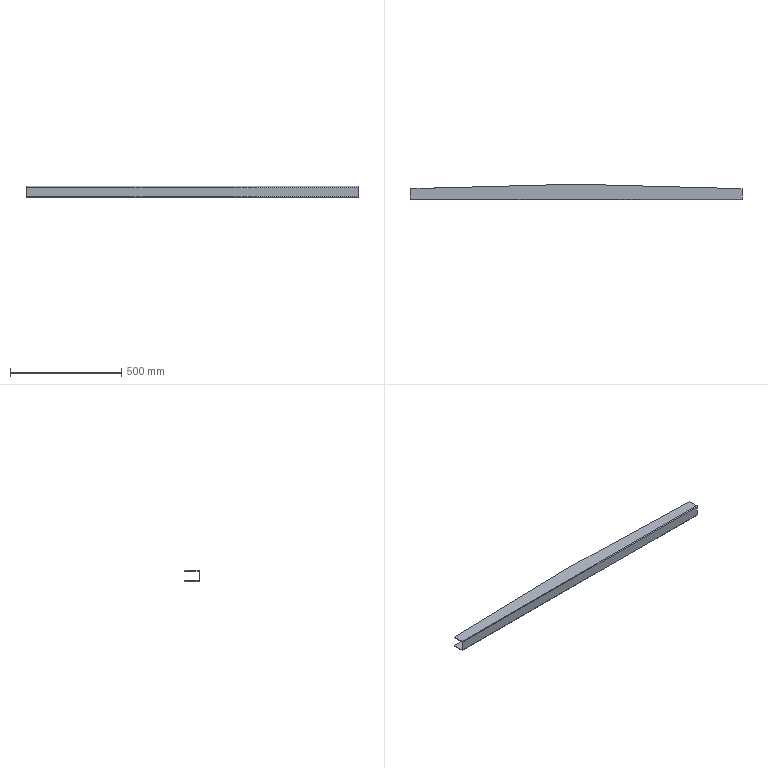Part | SolidWorks | 1 solid | 24 faces | box 1490 x 70 x 50 mm | volume 726941 mm3 | plane 20 | cylinder 4 | commonest cylinder face diameters 0.2 x2 6.2 x2
STEP:
#1=CARTESIAN_POINT('',(-745.,-3.,-21.9));
#2=VERTEX_POINT('',#1);
#3=CARTESIAN_POINT('',(745.,-3.,-21.9));
#4=VERTEX_POINT('',#3);
#5=CARTESIAN_POINT('',(-745.,-3.,-21.9));
#6=DIRECTION('',(1.,0.,0.));
#7=VECTOR('',#6,1000.);
#8=LINE('',#5,#7);
#9=EDGE_CURVE('',#2,#4,#8,.T.);
#10=ORIENTED_EDGE('',*,*,#9,.T.);
#11=CARTESIAN_POINT('',(745.,-3.,21.9));
#12=VERTEX_POINT('',#11);
#13=CARTESIAN_POINT('',(745.,-3.,25.));
#14=DIRECTION('',(0.,0.,-1.));
#15=VECTOR('',#14,1000.);
#16=LINE('',#13,#15);
#17=EDGE_CURVE('',#12,#4,#16,.T.);
#18=ORIENTED_EDGE('',*,*,#17,.F.);
#19=CARTESIAN_POINT('',(-745.,-3.,21.9));
#20=VERTEX_POINT('',#19);
#21=CARTESIAN_POINT('',(745.,-3.,21.9));
#22=DIRECTION('',(-1.,0.,0.));
#23=VECTOR('',#22,1000.);
#24=LINE('',#21,#23);
#25=EDGE_CURVE('',#12,#20,#24,.T.);
#26=ORIENTED_EDGE('',*,*,#25,.T.);
#27=CARTESIAN_POINT('',(-745.,-3.,25.));
#28=DIRECTION('',(0.,0.,1.));
#29=VECTOR('',#28,1000.);
#30=LINE('',#27,#29);
#31=EDGE_CURVE('',#2,#20,#30,.T.);
#32=ORIENTED_EDGE('',*,*,#31,.F.);
#33=EDGE_LOOP('',(#10,#18,#26,#32));
#34=FACE_OUTER_BOUND('',#33,.T.);
#35=CARTESIAN_POINT('',(0.,-3.,0.));
#36=DIRECTION('',(0.,1.,0.));
#37=DIRECTION('',(0.,0.,1.));
#38=AXIS2_PLACEMENT_3D('',#35,#36,#37);
#39=PLANE('',#38);
#40=ADVANCED_FACE('',(#34),#39,.F.);
#41=CARTESIAN_POINT('',(745.,0.,21.9));
#42=VERTEX_POINT('',#41);
#43=CARTESIAN_POINT('',(745.,0.,-21.9));
#44=VERTEX_POINT('',#43);
#45=CARTESIAN_POINT('',(745.,0.,25.));
#46=DIRECTION('',(0.,0.,-1.));
#47=VECTOR('',#46,1000.);
#48=LINE('',#45,#47);
#49=EDGE_CURVE('',#42,#44,#48,.T.);
#50=ORIENTED_EDGE('',*,*,#49,.T.);
#51=CARTESIAN_POINT('',(-745.,0.,-21.9));
#52=VERTEX_POINT('',#51);
#53=CARTESIAN_POINT('',(-745.,0.,-21.9));
#54=DIRECTION('',(1.,0.,0.));
#55=VECTOR('',#54,1000.);
#56=LINE('',#53,#55);
#57=EDGE_CURVE('',#52,#44,#56,.T.);
#58=ORIENTED_EDGE('',*,*,#57,.F.);
#59=CARTESIAN_POINT('',(-745.,0.,21.9));
#60=VERTEX_POINT('',#59);
#61=CARTESIAN_POINT('',(-745.,0.,25.));
#62=DIRECTION('',(0.,0.,1.));
#63=VECTOR('',#62,1000.);
#64=LINE('',#61,#63);
#65=EDGE_CURVE('',#52,#60,#64,.T.);
#66=ORIENTED_EDGE('',*,*,#65,.T.);
#67=CARTESIAN_POINT('',(745.,0.,21.9));
#68=DIRECTION('',(-1.,0.,0.));
#69=VECTOR('',#68,1000.);
#70=LINE('',#67,#69);
#71=EDGE_CURVE('',#42,#60,#70,.T.);
#72=ORIENTED_EDGE('',*,*,#71,.F.);
#73=EDGE_LOOP('',(#50,#58,#66,#72));
#74=FACE_OUTER_BOUND('',#73,.T.);
#75=CARTESIAN_POINT('',(0.,0.,0.));
#76=DIRECTION('',(0.,1.,0.));
#77=DIRECTION('',(0.,0.,1.));
#78=AXIS2_PLACEMENT_3D('',#75,#76,#77);
#79=PLANE('',#78);
#80=ADVANCED_FACE('',(#74),#79,.T.);
#81=ORIENTED_EDGE('',*,*,#65,.F.);
#82=CARTESIAN_POINT('',(-745.,0.,-21.9));
#83=DIRECTION('',(0.,-1.,0.));
#84=VECTOR('',#83,1000.);
#85=LINE('',#82,#84);
#86=EDGE_CURVE('',#52,#2,#85,.T.);
#87=ORIENTED_EDGE('',*,*,#86,.T.);
#88=ORIENTED_EDGE('',*,*,#31,.T.);
#89=CARTESIAN_POINT('',(-745.,0.,21.9));
#90=DIRECTION('',(0.,-1.,0.));
#91=VECTOR('',#90,1000.);
#92=LINE('',#89,#91);
#93=EDGE_CURVE('',#60,#20,#92,.T.);
#94=ORIENTED_EDGE('',*,*,#93,.F.);
#95=EDGE_LOOP('',(#81,#87,#88,#94));
#96=FACE_OUTER_BOUND('',#95,.T.);
#97=CARTESIAN_POINT('',(-745.,-3.,25.));
#98=DIRECTION('',(-1.,0.,0.));
#99=DIRECTION('',(0.,0.,1.));
#100=AXIS2_PLACEMENT_3D('',#97,#98,#99);
#101=PLANE('',#100);
#102=ADVANCED_FACE('',(#96),#101,.T.);
#103=CARTESIAN_POINT('',(745.,0.,-21.9));
#104=DIRECTION('',(0.,-1.,0.));
#105=VECTOR('',#104,1000.);
#106=LINE('',#103,#105);
#107=EDGE_CURVE('',#44,#4,#106,.T.);
#108=ORIENTED_EDGE('',*,*,#107,.F.);
#109=ORIENTED_EDGE('',*,*,#49,.F.);
#110=CARTESIAN_POINT('',(745.,0.,21.9));
#111=DIRECTION('',(0.,-1.,0.));
#112=VECTOR('',#111,1000.);
#113=LINE('',#110,#112);
#114=EDGE_CURVE('',#42,#12,#113,.T.);
#115=ORIENTED_EDGE('',*,*,#114,.T.);
#116=ORIENTED_EDGE('',*,*,#17,.T.);
#117=EDGE_LOOP('',(#108,#109,#115,#116));
#118=FACE_OUTER_BOUND('',#117,.T.);
#119=CARTESIAN_POINT('',(745.,-3.,25.));
#120=DIRECTION('',(1.,0.,0.));
#121=DIRECTION('',(0.,0.,-1.));
#122=AXIS2_PLACEMENT_3D('',#119,#120,#121);
#123=PLANE('',#122);
#124=ADVANCED_FACE('',(#118),#123,.T.);
#125=CARTESIAN_POINT('',(-745.,0.1,22.));
#126=VERTEX_POINT('',#125);
#127=CARTESIAN_POINT('',(-745.,0.1,25.));
#128=VERTEX_POINT('',#127);
#129=CARTESIAN_POINT('',(-745.,0.1,25.));
#130=DIRECTION('',(0.,0.,1.));
#131=VECTOR('',#130,1000.);
#132=LINE('',#129,#131);
#133=EDGE_CURVE('',#126,#128,#132,.T.);
#134=ORIENTED_EDGE('',*,*,#133,.F.);
#135=CARTESIAN_POINT('',(-745.,0.1,21.9));
#136=DIRECTION('',(-1.,0.,0.));
#137=DIRECTION('',(0.,0.,-1.));
#138=AXIS2_PLACEMENT_3D('',#135,#136,#137);
#139=CIRCLE('',#138,0.1);
#140=EDGE_CURVE('',#60,#126,#139,.T.);
#141=ORIENTED_EDGE('',*,*,#140,.F.);
#142=ORIENTED_EDGE('',*,*,#93,.T.);
#143=CARTESIAN_POINT('',(-745.,0.1,21.9));
#144=DIRECTION('',(-1.,0.,0.));
#145=DIRECTION('',(0.,0.,-1.));
#146=AXIS2_PLACEMENT_3D('',#143,#144,#145);
#147=CIRCLE('',#146,3.1);
#148=EDGE_CURVE('',#20,#128,#147,.T.);
#149=ORIENTED_EDGE('',*,*,#148,.T.);
#150=EDGE_LOOP('',(#134,#141,#142,#149));
#151=FACE_OUTER_BOUND('',#150,.T.);
#152=CARTESIAN_POINT('',(-745.,0.1,21.9));
#153=DIRECTION('',(-1.,0.,0.));
#154=DIRECTION('',(0.,0.,1.));
#155=AXIS2_PLACEMENT_3D('',#152,#153,#154);
#156=PLANE('',#155);
#157=ADVANCED_FACE('',(#151),#156,.T.);
#158=CARTESIAN_POINT('',(745.,0.1,22.));
#159=VERTEX_POINT('',#158);
#160=CARTESIAN_POINT('',(745.,0.1,21.9));
#161=DIRECTION('',(1.,0.,0.));
#162=DIRECTION('',(0.,0.,-1.));
#163=AXIS2_PLACEMENT_3D('',#160,#161,#162);
#164=CIRCLE('',#163,0.1);
#165=EDGE_CURVE('',#159,#42,#164,.T.);
#166=ORIENTED_EDGE('',*,*,#165,.F.);
#167=CARTESIAN_POINT('',(745.,0.1,25.));
#168=VERTEX_POINT('',#167);
#169=CARTESIAN_POINT('',(745.,0.1,22.));
#170=DIRECTION('',(0.,0.,1.));
#171=VECTOR('',#170,1000.);
#172=LINE('',#169,#171);
#173=EDGE_CURVE('',#159,#168,#172,.T.);
#174=ORIENTED_EDGE('',*,*,#173,.T.);
#175=CARTESIAN_POINT('',(745.,0.1,21.9));
#176=DIRECTION('',(1.,0.,0.));
#177=DIRECTION('',(0.,0.,-1.));
#178=AXIS2_PLACEMENT_3D('',#175,#176,#177);
#179=CIRCLE('',#178,3.1);
#180=EDGE_CURVE('',#168,#12,#179,.T.);
#181=ORIENTED_EDGE('',*,*,#180,.T.);
#182=ORIENTED_EDGE('',*,*,#114,.F.);
#183=EDGE_LOOP('',(#166,#174,#181,#182));
#184=FACE_OUTER_BOUND('',#183,.T.);
#185=CARTESIAN_POINT('',(745.,0.1,21.9));
#186=DIRECTION('',(-1.,0.,0.));
#187=DIRECTION('',(0.,0.,1.));
#188=AXIS2_PLACEMENT_3D('',#185,#186,#187);
#189=PLANE('',#188);
#190=ADVANCED_FACE('',(#184),#189,.F.);
#191=ORIENTED_EDGE('',*,*,#25,.F.);
#192=ORIENTED_EDGE('',*,*,#180,.F.);
#193=CARTESIAN_POINT('',(-745.,0.1,25.));
#194=DIRECTION('',(-1.,0.,0.));
#195=VECTOR('',#194,1000.);
#196=LINE('',#193,#195);
#197=EDGE_CURVE('',#168,#128,#196,.T.);
#198=ORIENTED_EDGE('',*,*,#197,.T.);
#199=ORIENTED_EDGE('',*,*,#148,.F.);
#200=EDGE_LOOP('',(#191,#192,#198,#199));
#201=FACE_OUTER_BOUND('',#200,.T.);
#202=CARTESIAN_POINT('',(745.,0.1,21.9));
#203=DIRECTION('',(1.,0.,0.));
#204=DIRECTION('',(0.,0.,1.));
#205=AXIS2_PLACEMENT_3D('',#202,#203,#204);
#206=CYLINDRICAL_SURFACE('',#205,3.1);
#207=ADVANCED_FACE('',(#201),#206,.T.);
#208=ORIENTED_EDGE('',*,*,#71,.T.);
#209=ORIENTED_EDGE('',*,*,#140,.T.);
#210=CARTESIAN_POINT('',(-745.,0.1,22.));
#211=DIRECTION('',(1.,0.,0.));
#212=VECTOR('',#211,1000.);
#213=LINE('',#210,#212);
#214=EDGE_CURVE('',#126,#159,#213,.T.);
#215=ORIENTED_EDGE('',*,*,#214,.T.);
#216=ORIENTED_EDGE('',*,*,#165,.T.);
#217=EDGE_LOOP('',(#208,#209,#215,#216));
#218=FACE_OUTER_BOUND('',#217,.T.);
#219=CARTESIAN_POINT('',(745.,0.1,21.9));
#220=DIRECTION('',(1.,0.,0.));
#221=DIRECTION('',(0.,0.,1.));
#222=AXIS2_PLACEMENT_3D('',#219,#220,#221);
#223=CYLINDRICAL_SURFACE('',#222,0.1);
#224=ADVANCED_FACE('',(#218),#223,.F.);
#225=ORIENTED_EDGE('',*,*,#133,.T.);
#226=CARTESIAN_POINT('',(-745.,47.,25.));
#227=VERTEX_POINT('',#226);
#228=CARTESIAN_POINT('',(-745.,0.,25.));
#229=DIRECTION('',(0.,-1.,0.));
#230=VECTOR('',#229,1000.);
#231=LINE('',#228,#230);
#232=EDGE_CURVE('',#227,#128,#231,.T.);
#233=ORIENTED_EDGE('',*,*,#232,.F.);
#234=CARTESIAN_POINT('',(-745.,47.,22.));
#235=VERTEX_POINT('',#234);
#236=CARTESIAN_POINT('',(-745.,47.,25.));
#237=DIRECTION('',(0.,0.,-1.));
#238=VECTOR('',#237,1000.);
#239=LINE('',#236,#238);
#240=EDGE_CURVE('',#227,#235,#239,.T.);
#241=ORIENTED_EDGE('',*,*,#240,.T.);
#242=CARTESIAN_POINT('',(-745.,0.,22.));
#243=DIRECTION('',(0.,-1.,0.));
#244=VECTOR('',#243,1000.);
#245=LINE('',#242,#244);
#246=EDGE_CURVE('',#235,#126,#245,.T.);
#247=ORIENTED_EDGE('',*,*,#246,.T.);
#248=EDGE_LOOP('',(#225,#233,#241,#247));
#249=FACE_OUTER_BOUND('',#248,.T.);
#250=CARTESIAN_POINT('',(-745.,0.,25.));
#251=DIRECTION('',(1.,0.,0.));
#252=DIRECTION('',(0.,0.,-1.));
#253=AXIS2_PLACEMENT_3D('',#250,#251,#252);
#254=PLANE('',#253);
#255=ADVANCED_FACE('',(#249),#254,.F.);
#256=ORIENTED_EDGE('',*,*,#173,.F.);
#257=CARTESIAN_POINT('',(745.,47.,22.));
#258=VERTEX_POINT('',#257);
#259=CARTESIAN_POINT('',(745.,47.,22.));
#260=DIRECTION('',(0.,1.,0.));
#261=VECTOR('',#260,1000.);
#262=LINE('',#259,#261);
#263=EDGE_CURVE('',#159,#258,#262,.T.);
#264=ORIENTED_EDGE('',*,*,#263,.T.);
#265=CARTESIAN_POINT('',(745.,47.,25.));
#266=VERTEX_POINT('',#265);
#267=CARTESIAN_POINT('',(745.,47.,25.));
#268=DIRECTION('',(0.,0.,-1.));
#269=VECTOR('',#268,1000.);
#270=LINE('',#267,#269);
#271=EDGE_CURVE('',#266,#258,#270,.T.);
#272=ORIENTED_EDGE('',*,*,#271,.F.);
#273=CARTESIAN_POINT('',(745.,0.,25.));
#274=DIRECTION('',(0.,1.,0.));
#275=VECTOR('',#274,1000.);
#276=LINE('',#273,#275);
#277=EDGE_CURVE('',#168,#266,#276,.T.);
#278=ORIENTED_EDGE('',*,*,#277,.F.);
#279=EDGE_LOOP('',(#256,#264,#272,#278));
#280=FACE_OUTER_BOUND('',#279,.T.);
#281=CARTESIAN_POINT('',(745.,47.,25.));
#282=DIRECTION('',(-1.,0.,0.));
#283=DIRECTION('',(0.,0.,1.));
#284=AXIS2_PLACEMENT_3D('',#281,#282,#283);
#285=PLANE('',#284);
#286=ADVANCED_FACE('',(#280),#285,.F.);
#287=ORIENTED_EDGE('',*,*,#197,.F.);
#288=ORIENTED_EDGE('',*,*,#277,.T.);
#289=CARTESIAN_POINT('',(0.,67.,25.));
#290=VERTEX_POINT('',#289);
#291=CARTESIAN_POINT('',(1.797,66.952,25.));
#292=DIRECTION('',(-0.9996,0.02684,0.));
#293=VECTOR('',#292,1000.);
#294=LINE('',#291,#293);
#295=EDGE_CURVE('',#266,#290,#294,.T.);
#296=ORIENTED_EDGE('',*,*,#295,.T.);
#297=CARTESIAN_POINT('',(-1.797,66.952,25.));
#298=DIRECTION('',(-0.9996,-0.02684,0.));
#299=VECTOR('',#298,1000.);
#300=LINE('',#297,#299);
#301=EDGE_CURVE('',#290,#227,#300,.T.);
#302=ORIENTED_EDGE('',*,*,#301,.T.);
#303=ORIENTED_EDGE('',*,*,#232,.T.);
#304=EDGE_LOOP('',(#287,#288,#296,#302,#303));
#305=FACE_OUTER_BOUND('',#304,.T.);
#306=CARTESIAN_POINT('',(0.,0.,25.));
#307=DIRECTION('',(0.,0.,-1.));
#308=DIRECTION('',(-1.,0.,0.));
#309=AXIS2_PLACEMENT_3D('',#306,#307,#308);
#310=PLANE('',#309);
#311=ADVANCED_FACE('',(#305),#310,.F.);
#312=ORIENTED_EDGE('',*,*,#263,.F.);
#313=ORIENTED_EDGE('',*,*,#214,.F.);
#314=ORIENTED_EDGE('',*,*,#246,.F.);
#315=CARTESIAN_POINT('',(0.,67.,22.));
#316=VERTEX_POINT('',#315);
#317=CARTESIAN_POINT('',(-745.,47.,22.));
#318=DIRECTION('',(-0.9996,-0.02684,0.));
#319=VECTOR('',#318,1000.);
#320=LINE('',#317,#319);
#321=EDGE_CURVE('',#316,#235,#320,.T.);
#322=ORIENTED_EDGE('',*,*,#321,.F.);
#323=CARTESIAN_POINT('',(0.,67.,22.));
#324=DIRECTION('',(-0.9996,0.02684,0.));
#325=VECTOR('',#324,1000.);
#326=LINE('',#323,#325);
#327=EDGE_CURVE('',#258,#316,#326,.T.);
#328=ORIENTED_EDGE('',*,*,#327,.F.);
#329=EDGE_LOOP('',(#312,#313,#314,#322,#328));
#330=FACE_OUTER_BOUND('',#329,.T.);
#331=CARTESIAN_POINT('',(0.,0.,22.));
#332=DIRECTION('',(0.,0.,-1.));
#333=DIRECTION('',(-1.,0.,0.));
#334=AXIS2_PLACEMENT_3D('',#331,#332,#333);
#335=PLANE('',#334);
#336=ADVANCED_FACE('',(#330),#335,.T.);
#337=ORIENTED_EDGE('',*,*,#327,.T.);
#338=CARTESIAN_POINT('',(0.,67.,25.));
#339=DIRECTION('',(0.,0.,-1.));
#340=VECTOR('',#339,1000.);
#341=LINE('',#338,#340);
#342=EDGE_CURVE('',#290,#316,#341,.T.);
#343=ORIENTED_EDGE('',*,*,#342,.F.);
#344=ORIENTED_EDGE('',*,*,#295,.F.);
#345=ORIENTED_EDGE('',*,*,#271,.T.);
#346=EDGE_LOOP('',(#337,#343,#344,#345));
#347=FACE_OUTER_BOUND('',#346,.T.);
#348=CARTESIAN_POINT('',(0.,67.,25.));
#349=DIRECTION('',(-0.02684,-0.9996,0.));
#350=DIRECTION('',(0.9996,-0.02684,0.));
#351=AXIS2_PLACEMENT_3D('',#348,#349,#350);
#352=PLANE('',#351);
#353=ADVANCED_FACE('',(#347),#352,.F.);
#354=ORIENTED_EDGE('',*,*,#321,.T.);
#355=ORIENTED_EDGE('',*,*,#240,.F.);
#356=ORIENTED_EDGE('',*,*,#301,.F.);
#357=ORIENTED_EDGE('',*,*,#342,.T.);
#358=EDGE_LOOP('',(#354,#355,#356,#357));
#359=FACE_OUTER_BOUND('',#358,.T.);
#360=CARTESIAN_POINT('',(-745.,47.,25.));
#361=DIRECTION('',(0.02684,-0.9996,0.));
#362=DIRECTION('',(0.9996,0.02684,0.));
#363=AXIS2_PLACEMENT_3D('',#360,#361,#362);
#364=PLANE('',#363);
#365=ADVANCED_FACE('',(#359),#364,.F.);
#366=CARTESIAN_POINT('',(745.,0.1,-22.));
#367=VERTEX_POINT('',#366);
#368=CARTESIAN_POINT('',(745.,0.1,-25.));
#369=VERTEX_POINT('',#368);
#370=CARTESIAN_POINT('',(745.,0.1,-25.));
#371=DIRECTION('',(0.,0.,-1.));
#372=VECTOR('',#371,1000.);
#373=LINE('',#370,#372);
#374=EDGE_CURVE('',#367,#369,#373,.T.);
#375=ORIENTED_EDGE('',*,*,#374,.F.);
#376=CARTESIAN_POINT('',(745.,0.1,-21.9));
#377=DIRECTION('',(1.,0.,0.));
#378=DIRECTION('',(0.,-1.,0.));
#379=AXIS2_PLACEMENT_3D('',#376,#377,#378);
#380=CIRCLE('',#379,0.1);
#381=EDGE_CURVE('',#44,#367,#380,.T.);
#382=ORIENTED_EDGE('',*,*,#381,.F.);
#383=ORIENTED_EDGE('',*,*,#107,.T.);
#384=CARTESIAN_POINT('',(745.,0.1,-21.9));
#385=DIRECTION('',(1.,0.,0.));
#386=DIRECTION('',(0.,-1.,0.));
#387=AXIS2_PLACEMENT_3D('',#384,#385,#386);
#388=CIRCLE('',#387,3.1);
#389=EDGE_CURVE('',#4,#369,#388,.T.);
#390=ORIENTED_EDGE('',*,*,#389,.T.);
#391=EDGE_LOOP('',(#375,#382,#383,#390));
#392=FACE_OUTER_BOUND('',#391,.T.);
#393=CARTESIAN_POINT('',(745.,0.1,-21.9));
#394=DIRECTION('',(1.,0.,0.));
#395=DIRECTION('',(0.,1.,0.));
#396=AXIS2_PLACEMENT_3D('',#393,#394,#395);
#397=PLANE('',#396);
#398=ADVANCED_FACE('',(#392),#397,.T.);
#399=CARTESIAN_POINT('',(-745.,0.1,-22.));
#400=VERTEX_POINT('',#399);
#401=CARTESIAN_POINT('',(-745.,0.1,-21.9));
#402=DIRECTION('',(-1.,0.,0.));
#403=DIRECTION('',(0.,-1.,0.));
#404=AXIS2_PLACEMENT_3D('',#401,#402,#403);
#405=CIRCLE('',#404,0.1);
#406=EDGE_CURVE('',#400,#52,#405,.T.);
#407=ORIENTED_EDGE('',*,*,#406,.F.);
#408=CARTESIAN_POINT('',(-745.,0.1,-25.));
#409=VERTEX_POINT('',#408);
#410=CARTESIAN_POINT('',(-745.,0.1,-22.));
#411=DIRECTION('',(0.,0.,-1.));
#412=VECTOR('',#411,1000.);
#413=LINE('',#410,#412);
#414=EDGE_CURVE('',#400,#409,#413,.T.);
#415=ORIENTED_EDGE('',*,*,#414,.T.);
#416=CARTESIAN_POINT('',(-745.,0.1,-21.9));
#417=DIRECTION('',(-1.,0.,0.));
#418=DIRECTION('',(0.,-1.,0.));
#419=AXIS2_PLACEMENT_3D('',#416,#417,#418);
#420=CIRCLE('',#419,3.1);
#421=EDGE_CURVE('',#409,#2,#420,.T.);
#422=ORIENTED_EDGE('',*,*,#421,.T.);
#423=ORIENTED_EDGE('',*,*,#86,.F.);
#424=EDGE_LOOP('',(#407,#415,#422,#423));
#425=FACE_OUTER_BOUND('',#424,.T.);
#426=CARTESIAN_POINT('',(-745.,0.1,-21.9));
#427=DIRECTION('',(1.,0.,0.));
#428=DIRECTION('',(0.,1.,0.));
#429=AXIS2_PLACEMENT_3D('',#426,#427,#428);
#430=PLANE('',#429);
#431=ADVANCED_FACE('',(#425),#430,.F.);
#432=ORIENTED_EDGE('',*,*,#9,.F.);
#433=ORIENTED_EDGE('',*,*,#421,.F.);
#434=CARTESIAN_POINT('',(745.,0.1,-25.));
#435=DIRECTION('',(1.,0.,0.));
#436=VECTOR('',#435,1000.);
#437=LINE('',#434,#436);
#438=EDGE_CURVE('',#409,#369,#437,.T.);
#439=ORIENTED_EDGE('',*,*,#438,.T.);
#440=ORIENTED_EDGE('',*,*,#389,.F.);
#441=EDGE_LOOP('',(#432,#433,#439,#440));
#442=FACE_OUTER_BOUND('',#441,.T.);
#443=CARTESIAN_POINT('',(-745.,0.1,-21.9));
#444=DIRECTION('',(-1.,0.,0.));
#445=DIRECTION('',(0.,0.,-1.));
#446=AXIS2_PLACEMENT_3D('',#443,#444,#445);
#447=CYLINDRICAL_SURFACE('',#446,3.1);
#448=ADVANCED_FACE('',(#442),#447,.T.);
#449=ORIENTED_EDGE('',*,*,#57,.T.);
#450=ORIENTED_EDGE('',*,*,#381,.T.);
#451=CARTESIAN_POINT('',(745.,0.1,-22.));
#452=DIRECTION('',(-1.,0.,0.));
#453=VECTOR('',#452,1000.);
#454=LINE('',#451,#453);
#455=EDGE_CURVE('',#367,#400,#454,.T.);
#456=ORIENTED_EDGE('',*,*,#455,.T.);
#457=ORIENTED_EDGE('',*,*,#406,.T.);
#458=EDGE_LOOP('',(#449,#450,#456,#457));
#459=FACE_OUTER_BOUND('',#458,.T.);
#460=CARTESIAN_POINT('',(-745.,0.1,-21.9));
#461=DIRECTION('',(-1.,0.,0.));
#462=DIRECTION('',(0.,0.,-1.));
#463=AXIS2_PLACEMENT_3D('',#460,#461,#462);
#464=CYLINDRICAL_SURFACE('',#463,0.1);
#465=ADVANCED_FACE('',(#459),#464,.F.);
#466=ORIENTED_EDGE('',*,*,#374,.T.);
#467=CARTESIAN_POINT('',(745.,47.,-25.));
#468=VERTEX_POINT('',#467);
#469=CARTESIAN_POINT('',(745.,0.,-25.));
#470=DIRECTION('',(0.,-1.,0.));
#471=VECTOR('',#470,1000.);
#472=LINE('',#469,#471);
#473=EDGE_CURVE('',#468,#369,#472,.T.);
#474=ORIENTED_EDGE('',*,*,#473,.F.);
#475=CARTESIAN_POINT('',(745.,47.,-22.));
#476=VERTEX_POINT('',#475);
#477=CARTESIAN_POINT('',(745.,47.,-25.));
#478=DIRECTION('',(0.,0.,1.));
#479=VECTOR('',#478,1000.);
#480=LINE('',#477,#479);
#481=EDGE_CURVE('',#468,#476,#480,.T.);
#482=ORIENTED_EDGE('',*,*,#481,.T.);
#483=CARTESIAN_POINT('',(745.,0.,-22.));
#484=DIRECTION('',(0.,-1.,0.));
#485=VECTOR('',#484,1000.);
#486=LINE('',#483,#485);
#487=EDGE_CURVE('',#476,#367,#486,.T.);
#488=ORIENTED_EDGE('',*,*,#487,.T.);
#489=EDGE_LOOP('',(#466,#474,#482,#488));
#490=FACE_OUTER_BOUND('',#489,.T.);
#491=CARTESIAN_POINT('',(745.,0.,-25.));
#492=DIRECTION('',(-1.,0.,0.));
#493=DIRECTION('',(0.,0.,1.));
#494=AXIS2_PLACEMENT_3D('',#491,#492,#493);
#495=PLANE('',#494);
#496=ADVANCED_FACE('',(#490),#495,.F.);
#497=ORIENTED_EDGE('',*,*,#414,.F.);
#498=CARTESIAN_POINT('',(-745.,47.,-22.));
#499=VERTEX_POINT('',#498);
#500=CARTESIAN_POINT('',(-745.,47.,-22.));
#501=DIRECTION('',(0.,1.,0.));
#502=VECTOR('',#501,1000.);
#503=LINE('',#500,#502);
#504=EDGE_CURVE('',#400,#499,#503,.T.);
#505=ORIENTED_EDGE('',*,*,#504,.T.);
#506=CARTESIAN_POINT('',(-745.,47.,-25.));
#507=VERTEX_POINT('',#506);
#508=CARTESIAN_POINT('',(-745.,47.,-25.));
#509=DIRECTION('',(0.,0.,1.));
#510=VECTOR('',#509,1000.);
#511=LINE('',#508,#510);
#512=EDGE_CURVE('',#507,#499,#511,.T.);
#513=ORIENTED_EDGE('',*,*,#512,.F.);
#514=CARTESIAN_POINT('',(-745.,0.,-25.));
#515=DIRECTION('',(0.,1.,0.));
#516=VECTOR('',#515,1000.);
#517=LINE('',#514,#516);
#518=EDGE_CURVE('',#409,#507,#517,.T.);
#519=ORIENTED_EDGE('',*,*,#518,.F.);
#520=EDGE_LOOP('',(#497,#505,#513,#519));
#521=FACE_OUTER_BOUND('',#520,.T.);
#522=CARTESIAN_POINT('',(-745.,47.,-25.));
#523=DIRECTION('',(1.,0.,0.));
#524=DIRECTION('',(0.,0.,-1.));
#525=AXIS2_PLACEMENT_3D('',#522,#523,#524);
#526=PLANE('',#525);
#527=ADVANCED_FACE('',(#521),#526,.F.);
#528=ORIENTED_EDGE('',*,*,#438,.F.);
#529=ORIENTED_EDGE('',*,*,#518,.T.);
#530=CARTESIAN_POINT('',(0.,67.,-25.));
#531=VERTEX_POINT('',#530);
#532=CARTESIAN_POINT('',(-1.797,66.952,-25.));
#533=DIRECTION('',(0.9996,0.02684,0.));
#534=VECTOR('',#533,1000.);
#535=LINE('',#532,#534);
#536=EDGE_CURVE('',#507,#531,#535,.T.);
#537=ORIENTED_EDGE('',*,*,#536,.T.);
#538=CARTESIAN_POINT('',(1.797,66.952,-25.));
#539=DIRECTION('',(0.9996,-0.02684,0.));
#540=VECTOR('',#539,1000.);
#541=LINE('',#538,#540);
#542=EDGE_CURVE('',#531,#468,#541,.T.);
#543=ORIENTED_EDGE('',*,*,#542,.T.);
#544=ORIENTED_EDGE('',*,*,#473,.T.);
#545=EDGE_LOOP('',(#528,#529,#537,#543,#544));
#546=FACE_OUTER_BOUND('',#545,.T.);
#547=CARTESIAN_POINT('',(0.,0.,-25.));
#548=DIRECTION('',(0.,0.,1.));
#549=DIRECTION('',(0.,-1.,0.));
#550=AXIS2_PLACEMENT_3D('',#547,#548,#549);
#551=PLANE('',#550);
#552=ADVANCED_FACE('',(#546),#551,.F.);
#553=ORIENTED_EDGE('',*,*,#504,.F.);
#554=ORIENTED_EDGE('',*,*,#455,.F.);
#555=ORIENTED_EDGE('',*,*,#487,.F.);
#556=CARTESIAN_POINT('',(0.,67.,-22.));
#557=VERTEX_POINT('',#556);
#558=CARTESIAN_POINT('',(745.,47.,-22.));
#559=DIRECTION('',(0.9996,-0.02684,0.));
#560=VECTOR('',#559,1000.);
#561=LINE('',#558,#560);
#562=EDGE_CURVE('',#557,#476,#561,.T.);
#563=ORIENTED_EDGE('',*,*,#562,.F.);
#564=CARTESIAN_POINT('',(0.,67.,-22.));
#565=DIRECTION('',(0.9996,0.02684,0.));
#566=VECTOR('',#565,1000.);
#567=LINE('',#564,#566);
#568=EDGE_CURVE('',#499,#557,#567,.T.);
#569=ORIENTED_EDGE('',*,*,#568,.F.);
#570=EDGE_LOOP('',(#553,#554,#555,#563,#569));
#571=FACE_OUTER_BOUND('',#570,.T.);
#572=CARTESIAN_POINT('',(0.,0.,-22.));
#573=DIRECTION('',(0.,0.,1.));
#574=DIRECTION('',(0.,-1.,0.));
#575=AXIS2_PLACEMENT_3D('',#572,#573,#574);
#576=PLANE('',#575);
#577=ADVANCED_FACE('',(#571),#576,.T.);
#578=ORIENTED_EDGE('',*,*,#568,.T.);
#579=CARTESIAN_POINT('',(0.,67.,-25.));
#580=DIRECTION('',(0.,0.,1.));
#581=VECTOR('',#580,1000.);
#582=LINE('',#579,#581);
#583=EDGE_CURVE('',#531,#557,#582,.T.);
#584=ORIENTED_EDGE('',*,*,#583,.F.);
#585=ORIENTED_EDGE('',*,*,#536,.F.);
#586=ORIENTED_EDGE('',*,*,#512,.T.);
#587=EDGE_LOOP('',(#578,#584,#585,#586));
#588=FACE_OUTER_BOUND('',#587,.T.);
#589=CARTESIAN_POINT('',(0.,67.,-25.));
#590=DIRECTION('',(0.02684,-0.9996,0.));
#591=DIRECTION('',(0.9996,0.02684,0.));
#592=AXIS2_PLACEMENT_3D('',#589,#590,#591);
#593=PLANE('',#592);
#594=ADVANCED_FACE('',(#588),#593,.F.);
#595=ORIENTED_EDGE('',*,*,#562,.T.);
#596=ORIENTED_EDGE('',*,*,#481,.F.);
#597=ORIENTED_EDGE('',*,*,#542,.F.);
#598=ORIENTED_EDGE('',*,*,#583,.T.);
#599=EDGE_LOOP('',(#595,#596,#597,#598));
#600=FACE_OUTER_BOUND('',#599,.T.);
#601=CARTESIAN_POINT('',(745.,47.,-25.));
#602=DIRECTION('',(-0.02684,-0.9996,0.));
#603=DIRECTION('',(0.9996,-0.02684,0.));
#604=AXIS2_PLACEMENT_3D('',#601,#602,#603);
#605=PLANE('',#604);
#606=ADVANCED_FACE('',(#600),#605,.F.);
#607=CLOSED_SHELL('',(#40,#80,#102,#124,#157,#190,#207,#224,#255,#286,#311,#336,#353,#365,#398,#431,#448,#465,#496,#527,#552,#577,#594,#606));
#608=MANIFOLD_SOLID_BREP('',#607);
#609=CARTESIAN_POINT('',(0.,0.,0.));
#610=DIRECTION('',(0.,0.,1.));
#611=DIRECTION('',(1.,0.,0.));
#612=AXIS2_PLACEMENT_3D('',#609,#610,#611);
#613=(LENGTH_UNIT()NAMED_UNIT(*)SI_UNIT(.MILLI.,.METRE.));
#614=UNCERTAINTY_MEASURE_WITH_UNIT(LENGTH_MEASURE(0.00001),#613,'','');
#615=(NAMED_UNIT(*)PLANE_ANGLE_UNIT()SI_UNIT($,.RADIAN.));
#616=(NAMED_UNIT(*)SI_UNIT($,.STERADIAN.)SOLID_ANGLE_UNIT());
#617=(GEOMETRIC_REPRESENTATION_CONTEXT(3)GLOBAL_UNCERTAINTY_ASSIGNED_CONTEXT((#614))GLOBAL_UNIT_ASSIGNED_CONTEXT((#613,#615,#616))REPRESENTATION_CONTEXT('',''));
#618=ADVANCED_BREP_SHAPE_REPRESENTATION('',(#608,#612),#617);